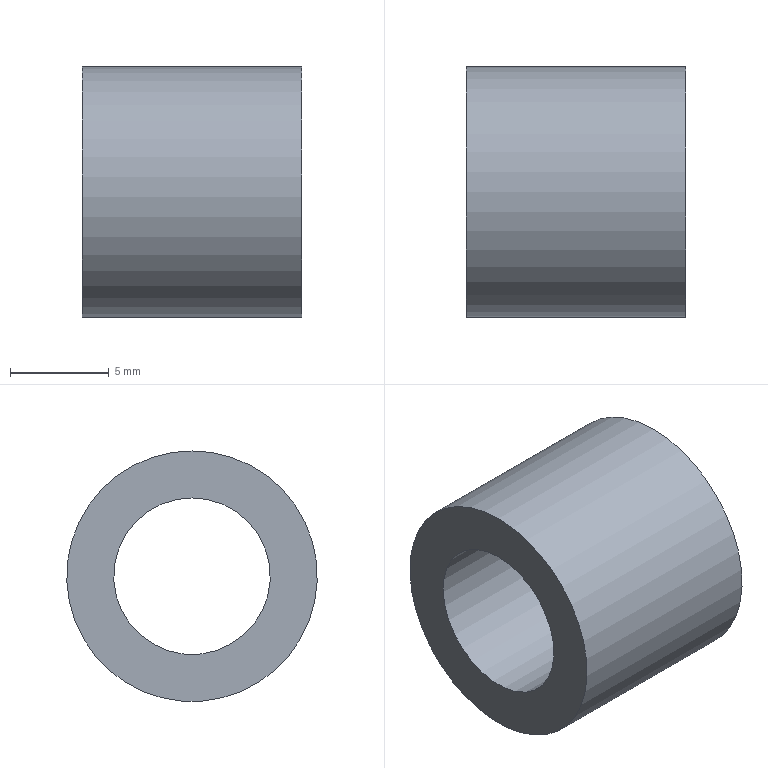Part | NX | features MG0318 steering bushings 2 | 1 solid | 4 faces | box 11.113 x 12.7 x 12.7 mm | volume 857.815 mm3 | plane 2 | cylinder 2 | commonest cylinder face diameters 7.938 x1 12.7 x1
STEP:
#1=CARTESIAN_POINT('',(0.,0.,3.969));
#2=VERTEX_POINT('',#1);
#3=CARTESIAN_POINT('',(0.,0.,0.));
#4=DIRECTION('',(-1.,0.,0.));
#5=DIRECTION('',(0.,0.,1.));
#6=AXIS2_PLACEMENT_3D('',#3,#4,#5);
#7=CIRCLE('',#6,3.969);
#8=EDGE_CURVE('',#2,#2,#7,.T.);
#9=ORIENTED_EDGE('',*,*,#8,.F.);
#10=EDGE_LOOP('',(#9));
#11=FACE_BOUND('',#10,.T.);
#12=CARTESIAN_POINT('',(0.,0.,6.35));
#13=VERTEX_POINT('',#12);
#14=CARTESIAN_POINT('',(0.,0.,0.));
#15=DIRECTION('',(-1.,0.,0.));
#16=DIRECTION('',(0.,0.,1.));
#17=AXIS2_PLACEMENT_3D('',#14,#15,#16);
#18=CIRCLE('',#17,6.35);
#19=EDGE_CURVE('',#13,#13,#18,.T.);
#20=ORIENTED_EDGE('',*,*,#19,.T.);
#21=EDGE_LOOP('',(#20));
#22=FACE_BOUND('',#21,.T.);
#23=CARTESIAN_POINT('',(0.,3.969,0.));
#24=DIRECTION('',(1.,0.,0.));
#25=DIRECTION('',(0.,0.,-1.));
#26=AXIS2_PLACEMENT_3D('',#23,#24,#25);
#27=PLANE('',#26);
#28=ADVANCED_FACE('',(#11,#22),#27,.F.);
#29=ORIENTED_EDGE('',*,*,#19,.F.);
#30=EDGE_LOOP('',(#29));
#31=FACE_BOUND('',#30,.T.);
#32=CARTESIAN_POINT('',(11.113,0.,6.35));
#33=VERTEX_POINT('',#32);
#34=CARTESIAN_POINT('',(11.113,0.,0.));
#35=DIRECTION('',(-1.,0.,0.));
#36=DIRECTION('',(0.,0.,1.));
#37=AXIS2_PLACEMENT_3D('',#34,#35,#36);
#38=CIRCLE('',#37,6.35);
#39=EDGE_CURVE('',#33,#33,#38,.T.);
#40=ORIENTED_EDGE('',*,*,#39,.T.);
#41=EDGE_LOOP('',(#40));
#42=FACE_BOUND('',#41,.T.);
#43=CARTESIAN_POINT('',(0.,0.,0.));
#44=DIRECTION('',(-1.,0.,0.));
#45=DIRECTION('',(0.,0.,1.));
#46=AXIS2_PLACEMENT_3D('',#43,#44,#45);
#47=CYLINDRICAL_SURFACE('',#46,6.35);
#48=ADVANCED_FACE('',(#31,#42),#47,.T.);
#49=ORIENTED_EDGE('',*,*,#39,.F.);
#50=EDGE_LOOP('',(#49));
#51=FACE_BOUND('',#50,.T.);
#52=CARTESIAN_POINT('',(11.113,0.,3.969));
#53=VERTEX_POINT('',#52);
#54=CARTESIAN_POINT('',(11.113,0.,0.));
#55=DIRECTION('',(-1.,0.,0.));
#56=DIRECTION('',(0.,0.,1.));
#57=AXIS2_PLACEMENT_3D('',#54,#55,#56);
#58=CIRCLE('',#57,3.969);
#59=EDGE_CURVE('',#53,#53,#58,.T.);
#60=ORIENTED_EDGE('',*,*,#59,.T.);
#61=EDGE_LOOP('',(#60));
#62=FACE_BOUND('',#61,.T.);
#63=CARTESIAN_POINT('',(11.113,3.969,0.));
#64=DIRECTION('',(-1.,0.,0.));
#65=DIRECTION('',(0.,0.,1.));
#66=AXIS2_PLACEMENT_3D('',#63,#64,#65);
#67=PLANE('',#66);
#68=ADVANCED_FACE('',(#51,#62),#67,.F.);
#69=ORIENTED_EDGE('',*,*,#59,.F.);
#70=EDGE_LOOP('',(#69));
#71=FACE_BOUND('',#70,.T.);
#72=ORIENTED_EDGE('',*,*,#8,.T.);
#73=EDGE_LOOP('',(#72));
#74=FACE_BOUND('',#73,.T.);
#75=CARTESIAN_POINT('',(0.,0.,0.));
#76=DIRECTION('',(-1.,0.,0.));
#77=DIRECTION('',(0.,0.,1.));
#78=AXIS2_PLACEMENT_3D('',#75,#76,#77);
#79=CYLINDRICAL_SURFACE('',#78,3.969);
#80=ADVANCED_FACE('',(#71,#74),#79,.F.);
#81=CLOSED_SHELL('',(#28,#48,#68,#80));
#82=MANIFOLD_SOLID_BREP('',#81);
#83=(LENGTH_UNIT()NAMED_UNIT(*)SI_UNIT(.MILLI.,.METRE.));
#84=UNCERTAINTY_MEASURE_WITH_UNIT(LENGTH_MEASURE(0.00001),#83,'','');
#85=(NAMED_UNIT(*)PLANE_ANGLE_UNIT()SI_UNIT($,.RADIAN.));
#86=(NAMED_UNIT(*)SI_UNIT($,.STERADIAN.)SOLID_ANGLE_UNIT());
#87=(GEOMETRIC_REPRESENTATION_CONTEXT(3)GLOBAL_UNCERTAINTY_ASSIGNED_CONTEXT((#84))GLOBAL_UNIT_ASSIGNED_CONTEXT((#83,#85,#86))REPRESENTATION_CONTEXT('',''));
#88=ADVANCED_BREP_SHAPE_REPRESENTATION('',(#82),#87);